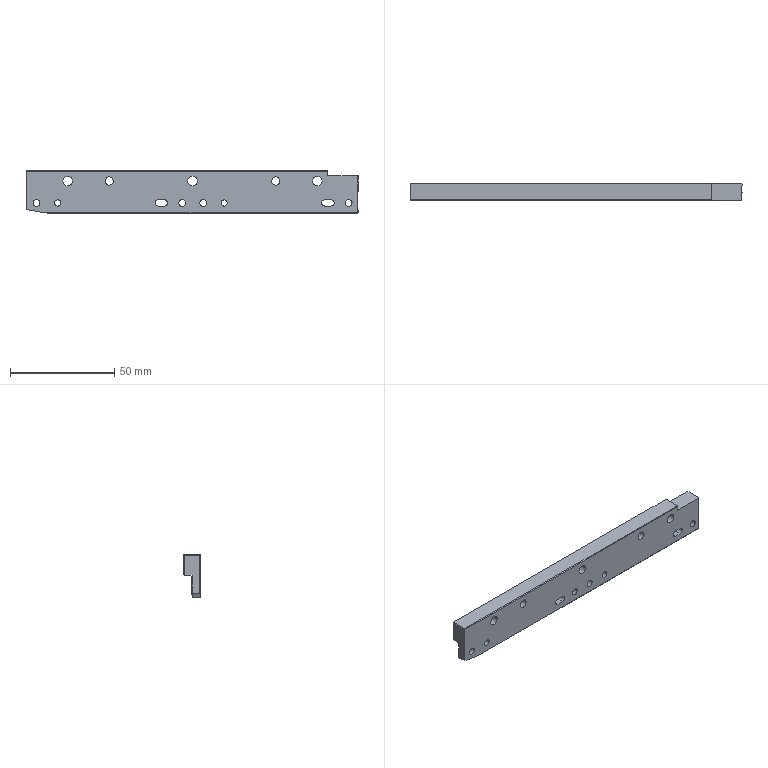Part | NX | 1 solid | 71 faces | box 159.5 x 8 x 20.5 mm | volume 18189 mm3 | cylinder 28 | plane 25 | cone 18 | commonest cylinder face diameters 3 x10 3.3 x8 4.5 x6 4 x4